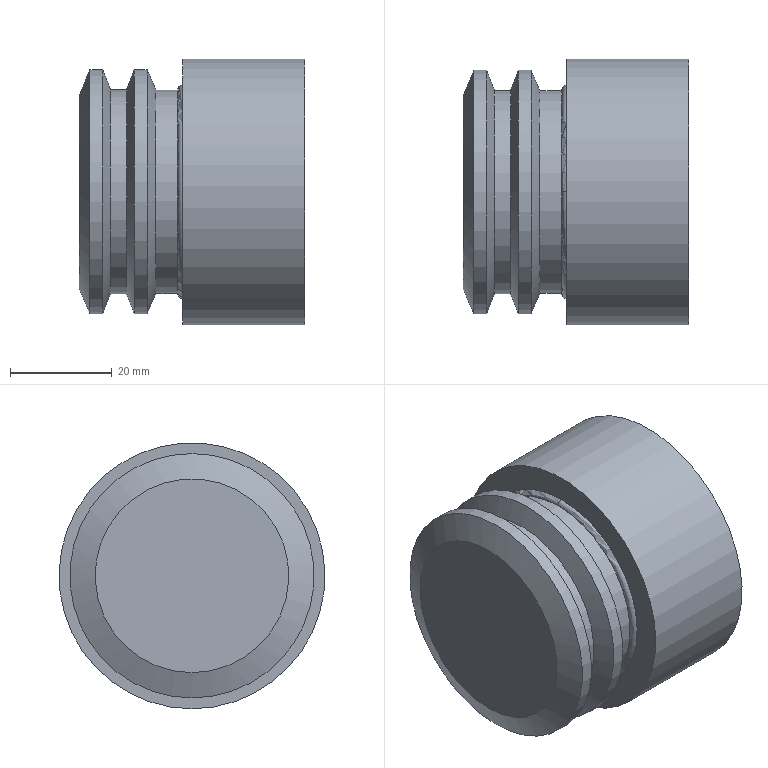Part | NX | features BREP 3 | 3 solids | 144 faces | box 44.35 x 52.257 x 52.257 mm | volume 61589 mm3 | torus 48 | cone 40 | cylinder 39 | plane 17 | commonest cylinder face diameters 24.45 x8 20.4 x4 22.02 x4 24.19 x4 32.55 x4 35.52 x4